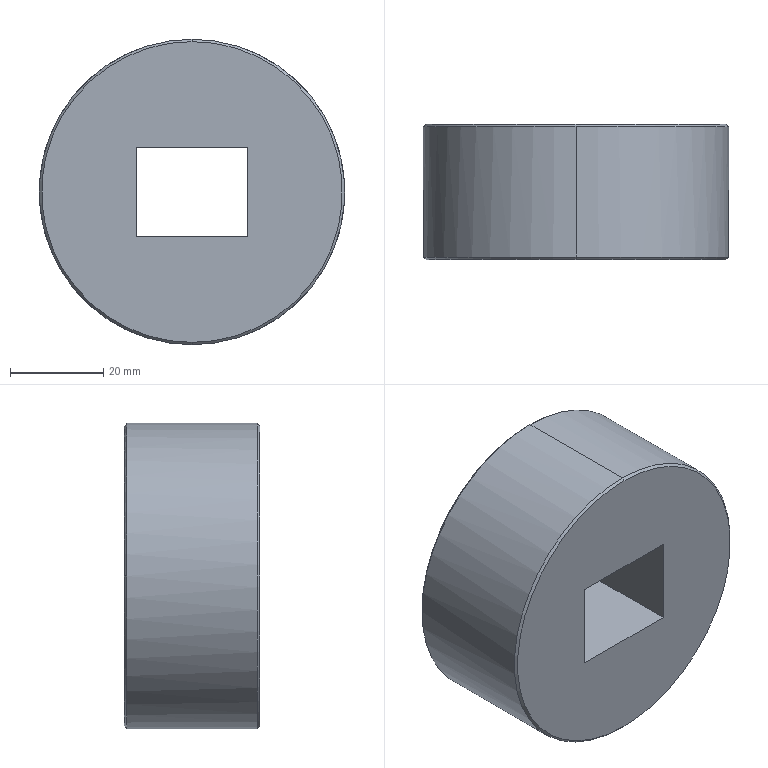Part | STEP file | _X2_4e007ea751859f7f5708_X0_MFB060_2.STEP.STEP | 1 solid | 12 faces | box 65.5 x 29 x 65.5 mm | volume 84346 mm3 | plane 6 | cone 4 | cylinder 2 | commonest cylinder face diameters 65.5 x2
STEP:
#1=CARTESIAN_POINT('',(32.75,28.5,0.));
#2=VERTEX_POINT('',#1);
#3=CARTESIAN_POINT('',(0.,28.5,32.75));
#4=VERTEX_POINT('',#3);
#5=CARTESIAN_POINT('',(0.,28.5,0.));
#6=DIRECTION('',(0.,-1.,0.));
#7=DIRECTION('',(0.,0.,-1.));
#8=AXIS2_PLACEMENT_3D('',#5,#6,#7);
#9=CIRCLE('',#8,32.75);
#10=EDGE_CURVE('',#2,#4,#9,.T.);
#11=ORIENTED_EDGE('',*,*,#10,.T.);
#12=CARTESIAN_POINT('',(0.,0.5,32.75));
#13=VERTEX_POINT('',#12);
#14=CARTESIAN_POINT('',(0.,29.,32.75));
#15=DIRECTION('',(0.,-1.,0.));
#16=VECTOR('',#15,1000.);
#17=LINE('',#14,#16);
#18=EDGE_CURVE('',#4,#13,#17,.T.);
#19=ORIENTED_EDGE('',*,*,#18,.T.);
#20=CARTESIAN_POINT('',(0.,0.5,-32.75));
#21=VERTEX_POINT('',#20);
#22=CARTESIAN_POINT('',(0.,0.5,0.));
#23=DIRECTION('',(0.,1.,0.));
#24=DIRECTION('',(0.,0.,-1.));
#25=AXIS2_PLACEMENT_3D('',#22,#23,#24);
#26=CIRCLE('',#25,32.75);
#27=EDGE_CURVE('',#13,#21,#26,.T.);
#28=ORIENTED_EDGE('',*,*,#27,.T.);
#29=CARTESIAN_POINT('',(0.,28.5,-32.75));
#30=VERTEX_POINT('',#29);
#31=CARTESIAN_POINT('',(0.,29.,-32.75));
#32=DIRECTION('',(0.,-1.,0.));
#33=VECTOR('',#32,1000.);
#34=LINE('',#31,#33);
#35=EDGE_CURVE('',#30,#21,#34,.T.);
#36=ORIENTED_EDGE('',*,*,#35,.F.);
#37=CARTESIAN_POINT('',(0.,28.5,0.));
#38=DIRECTION('',(0.,-1.,0.));
#39=DIRECTION('',(0.,0.,-1.));
#40=AXIS2_PLACEMENT_3D('',#37,#38,#39);
#41=CIRCLE('',#40,32.75);
#42=EDGE_CURVE('',#30,#2,#41,.T.);
#43=ORIENTED_EDGE('',*,*,#42,.T.);
#44=EDGE_LOOP('',(#11,#19,#28,#36,#43));
#45=FACE_OUTER_BOUND('',#44,.T.);
#46=CARTESIAN_POINT('',(0.,29.,0.));
#47=DIRECTION('',(0.,-1.,0.));
#48=DIRECTION('',(0.,0.,-1.));
#49=AXIS2_PLACEMENT_3D('',#46,#47,#48);
#50=CYLINDRICAL_SURFACE('',#49,32.75);
#51=ADVANCED_FACE('',(#45),#50,.T.);
#52=CARTESIAN_POINT('',(0.,0.,32.25));
#53=VERTEX_POINT('',#52);
#54=CARTESIAN_POINT('',(0.,0.,-32.25));
#55=VERTEX_POINT('',#54);
#56=CARTESIAN_POINT('',(0.,0.,0.));
#57=DIRECTION('',(0.,1.,0.));
#58=DIRECTION('',(0.,0.,1.));
#59=AXIS2_PLACEMENT_3D('',#56,#57,#58);
#60=CIRCLE('',#59,32.25);
#61=EDGE_CURVE('',#53,#55,#60,.T.);
#62=ORIENTED_EDGE('',*,*,#61,.T.);
#63=CARTESIAN_POINT('',(0.,0.5,-32.75));
#64=DIRECTION('',(0.,0.7071,-0.7071));
#65=VECTOR('',#64,1000.);
#66=LINE('',#63,#65);
#67=EDGE_CURVE('',#55,#21,#66,.T.);
#68=ORIENTED_EDGE('',*,*,#67,.T.);
#69=ORIENTED_EDGE('',*,*,#27,.F.);
#70=CARTESIAN_POINT('',(0.,0.5,32.75));
#71=DIRECTION('',(0.,0.7071,0.7071));
#72=VECTOR('',#71,1000.);
#73=LINE('',#70,#72);
#74=EDGE_CURVE('',#53,#13,#73,.T.);
#75=ORIENTED_EDGE('',*,*,#74,.F.);
#76=EDGE_LOOP('',(#62,#68,#69,#75));
#77=FACE_OUTER_BOUND('',#76,.T.);
#78=CARTESIAN_POINT('',(0.,0.5,0.));
#79=DIRECTION('',(0.,1.,0.));
#80=DIRECTION('',(0.,0.,1.));
#81=AXIS2_PLACEMENT_3D('',#78,#79,#80);
#82=CONICAL_SURFACE('',#81,32.75,0.7854);
#83=ADVANCED_FACE('',(#77),#82,.T.);
#84=CARTESIAN_POINT('',(32.25,29.,0.));
#85=VERTEX_POINT('',#84);
#86=CARTESIAN_POINT('',(-32.25,29.,0.));
#87=VERTEX_POINT('',#86);
#88=CARTESIAN_POINT('',(0.,29.,0.));
#89=DIRECTION('',(0.,-1.,0.));
#90=DIRECTION('',(1.,0.,0.));
#91=AXIS2_PLACEMENT_3D('',#88,#89,#90);
#92=CIRCLE('',#91,32.25);
#93=EDGE_CURVE('',#85,#87,#92,.T.);
#94=ORIENTED_EDGE('',*,*,#93,.T.);
#95=CARTESIAN_POINT('',(-32.75,28.5,0.));
#96=VERTEX_POINT('',#95);
#97=CARTESIAN_POINT('',(-32.75,28.5,0.));
#98=DIRECTION('',(-0.7071,-0.7071,0.));
#99=VECTOR('',#98,1000.);
#100=LINE('',#97,#99);
#101=EDGE_CURVE('',#87,#96,#100,.T.);
#102=ORIENTED_EDGE('',*,*,#101,.T.);
#103=CARTESIAN_POINT('',(0.,28.5,0.));
#104=DIRECTION('',(0.,-1.,0.));
#105=DIRECTION('',(0.,0.,-1.));
#106=AXIS2_PLACEMENT_3D('',#103,#104,#105);
#107=CIRCLE('',#106,32.75);
#108=EDGE_CURVE('',#4,#96,#107,.T.);
#109=ORIENTED_EDGE('',*,*,#108,.F.);
#110=ORIENTED_EDGE('',*,*,#10,.F.);
#111=CARTESIAN_POINT('',(32.75,28.5,0.));
#112=DIRECTION('',(0.7071,-0.7071,0.));
#113=VECTOR('',#112,1000.);
#114=LINE('',#111,#113);
#115=EDGE_CURVE('',#85,#2,#114,.T.);
#116=ORIENTED_EDGE('',*,*,#115,.F.);
#117=EDGE_LOOP('',(#94,#102,#109,#110,#116));
#118=FACE_OUTER_BOUND('',#117,.T.);
#119=CARTESIAN_POINT('',(0.,28.5,0.));
#120=DIRECTION('',(0.,-1.,0.));
#121=DIRECTION('',(1.,0.,0.));
#122=AXIS2_PLACEMENT_3D('',#119,#120,#121);
#123=CONICAL_SURFACE('',#122,32.75,0.7854);
#124=ADVANCED_FACE('',(#118),#123,.T.);
#125=ORIENTED_EDGE('',*,*,#18,.F.);
#126=ORIENTED_EDGE('',*,*,#108,.T.);
#127=CARTESIAN_POINT('',(0.,28.5,0.));
#128=DIRECTION('',(0.,-1.,0.));
#129=DIRECTION('',(0.,0.,-1.));
#130=AXIS2_PLACEMENT_3D('',#127,#128,#129);
#131=CIRCLE('',#130,32.75);
#132=EDGE_CURVE('',#96,#30,#131,.T.);
#133=ORIENTED_EDGE('',*,*,#132,.T.);
#134=ORIENTED_EDGE('',*,*,#35,.T.);
#135=CARTESIAN_POINT('',(0.,0.5,0.));
#136=DIRECTION('',(0.,1.,0.));
#137=DIRECTION('',(0.,0.,-1.));
#138=AXIS2_PLACEMENT_3D('',#135,#136,#137);
#139=CIRCLE('',#138,32.75);
#140=EDGE_CURVE('',#21,#13,#139,.T.);
#141=ORIENTED_EDGE('',*,*,#140,.T.);
#142=EDGE_LOOP('',(#125,#126,#133,#134,#141));
#143=FACE_OUTER_BOUND('',#142,.T.);
#144=CARTESIAN_POINT('',(0.,29.,0.));
#145=DIRECTION('',(0.,-1.,0.));
#146=DIRECTION('',(0.,0.,-1.));
#147=AXIS2_PLACEMENT_3D('',#144,#145,#146);
#148=CYLINDRICAL_SURFACE('',#147,32.75);
#149=ADVANCED_FACE('',(#143),#148,.T.);
#150=ORIENTED_EDGE('',*,*,#67,.F.);
#151=CARTESIAN_POINT('',(0.,0.,0.));
#152=DIRECTION('',(0.,1.,0.));
#153=DIRECTION('',(0.,0.,1.));
#154=AXIS2_PLACEMENT_3D('',#151,#152,#153);
#155=CIRCLE('',#154,32.25);
#156=EDGE_CURVE('',#55,#53,#155,.T.);
#157=ORIENTED_EDGE('',*,*,#156,.T.);
#158=ORIENTED_EDGE('',*,*,#74,.T.);
#159=ORIENTED_EDGE('',*,*,#140,.F.);
#160=EDGE_LOOP('',(#150,#157,#158,#159));
#161=FACE_OUTER_BOUND('',#160,.T.);
#162=CARTESIAN_POINT('',(0.,0.5,0.));
#163=DIRECTION('',(0.,1.,0.));
#164=DIRECTION('',(0.,0.,1.));
#165=AXIS2_PLACEMENT_3D('',#162,#163,#164);
#166=CONICAL_SURFACE('',#165,32.75,0.7854);
#167=ADVANCED_FACE('',(#161),#166,.T.);
#168=ORIENTED_EDGE('',*,*,#101,.F.);
#169=CARTESIAN_POINT('',(0.,29.,0.));
#170=DIRECTION('',(0.,-1.,0.));
#171=DIRECTION('',(1.,0.,0.));
#172=AXIS2_PLACEMENT_3D('',#169,#170,#171);
#173=CIRCLE('',#172,32.25);
#174=EDGE_CURVE('',#87,#85,#173,.T.);
#175=ORIENTED_EDGE('',*,*,#174,.T.);
#176=ORIENTED_EDGE('',*,*,#115,.T.);
#177=ORIENTED_EDGE('',*,*,#42,.F.);
#178=ORIENTED_EDGE('',*,*,#132,.F.);
#179=EDGE_LOOP('',(#168,#175,#176,#177,#178));
#180=FACE_OUTER_BOUND('',#179,.T.);
#181=CARTESIAN_POINT('',(0.,28.5,0.));
#182=DIRECTION('',(0.,-1.,0.));
#183=DIRECTION('',(1.,0.,0.));
#184=AXIS2_PLACEMENT_3D('',#181,#182,#183);
#185=CONICAL_SURFACE('',#184,32.75,0.7854);
#186=ADVANCED_FACE('',(#180),#185,.T.);
#187=ORIENTED_EDGE('',*,*,#61,.F.);
#188=ORIENTED_EDGE('',*,*,#156,.F.);
#189=EDGE_LOOP('',(#187,#188));
#190=FACE_OUTER_BOUND('',#189,.T.);
#191=CARTESIAN_POINT('',(11.93,0.,-9.625));
#192=VERTEX_POINT('',#191);
#193=CARTESIAN_POINT('',(11.93,0.,9.625));
#194=VERTEX_POINT('',#193);
#195=CARTESIAN_POINT('',(11.93,0.,0.));
#196=DIRECTION('',(0.,0.,1.));
#197=VECTOR('',#196,1000.);
#198=LINE('',#195,#197);
#199=EDGE_CURVE('',#192,#194,#198,.T.);
#200=ORIENTED_EDGE('',*,*,#199,.F.);
#201=CARTESIAN_POINT('',(-11.93,0.,-9.625));
#202=VERTEX_POINT('',#201);
#203=CARTESIAN_POINT('',(0.,0.,-9.625));
#204=DIRECTION('',(1.,0.,0.));
#205=VECTOR('',#204,1000.);
#206=LINE('',#203,#205);
#207=EDGE_CURVE('',#202,#192,#206,.T.);
#208=ORIENTED_EDGE('',*,*,#207,.F.);
#209=CARTESIAN_POINT('',(-11.93,0.,9.625));
#210=VERTEX_POINT('',#209);
#211=CARTESIAN_POINT('',(-11.93,0.,0.));
#212=DIRECTION('',(0.,0.,-1.));
#213=VECTOR('',#212,1000.);
#214=LINE('',#211,#213);
#215=EDGE_CURVE('',#210,#202,#214,.T.);
#216=ORIENTED_EDGE('',*,*,#215,.F.);
#217=CARTESIAN_POINT('',(0.,0.,9.625));
#218=DIRECTION('',(-1.,0.,0.));
#219=VECTOR('',#218,1000.);
#220=LINE('',#217,#219);
#221=EDGE_CURVE('',#194,#210,#220,.T.);
#222=ORIENTED_EDGE('',*,*,#221,.F.);
#223=EDGE_LOOP('',(#200,#208,#216,#222));
#224=FACE_BOUND('',#223,.T.);
#225=CARTESIAN_POINT('',(0.,0.,0.));
#226=DIRECTION('',(0.,1.,0.));
#227=DIRECTION('',(0.,0.,1.));
#228=AXIS2_PLACEMENT_3D('',#225,#226,#227);
#229=PLANE('',#228);
#230=ADVANCED_FACE('',(#190,#224),#229,.F.);
#231=ORIENTED_EDGE('',*,*,#93,.F.);
#232=ORIENTED_EDGE('',*,*,#174,.F.);
#233=EDGE_LOOP('',(#231,#232));
#234=FACE_OUTER_BOUND('',#233,.T.);
#235=CARTESIAN_POINT('',(-11.93,29.,9.625));
#236=VERTEX_POINT('',#235);
#237=CARTESIAN_POINT('',(-11.93,29.,-9.625));
#238=VERTEX_POINT('',#237);
#239=CARTESIAN_POINT('',(-11.93,29.,0.));
#240=DIRECTION('',(0.,0.,-1.));
#241=VECTOR('',#240,1000.);
#242=LINE('',#239,#241);
#243=EDGE_CURVE('',#236,#238,#242,.T.);
#244=ORIENTED_EDGE('',*,*,#243,.T.);
#245=CARTESIAN_POINT('',(11.93,29.,-9.625));
#246=VERTEX_POINT('',#245);
#247=CARTESIAN_POINT('',(0.,29.,-9.625));
#248=DIRECTION('',(1.,0.,0.));
#249=VECTOR('',#248,1000.);
#250=LINE('',#247,#249);
#251=EDGE_CURVE('',#238,#246,#250,.T.);
#252=ORIENTED_EDGE('',*,*,#251,.T.);
#253=CARTESIAN_POINT('',(11.93,29.,9.625));
#254=VERTEX_POINT('',#253);
#255=CARTESIAN_POINT('',(11.93,29.,0.));
#256=DIRECTION('',(0.,0.,1.));
#257=VECTOR('',#256,1000.);
#258=LINE('',#255,#257);
#259=EDGE_CURVE('',#246,#254,#258,.T.);
#260=ORIENTED_EDGE('',*,*,#259,.T.);
#261=CARTESIAN_POINT('',(0.,29.,9.625));
#262=DIRECTION('',(-1.,0.,0.));
#263=VECTOR('',#262,1000.);
#264=LINE('',#261,#263);
#265=EDGE_CURVE('',#254,#236,#264,.T.);
#266=ORIENTED_EDGE('',*,*,#265,.T.);
#267=EDGE_LOOP('',(#244,#252,#260,#266));
#268=FACE_BOUND('',#267,.T.);
#269=CARTESIAN_POINT('',(0.,29.,0.));
#270=DIRECTION('',(0.,1.,0.));
#271=DIRECTION('',(0.,0.,1.));
#272=AXIS2_PLACEMENT_3D('',#269,#270,#271);
#273=PLANE('',#272);
#274=ADVANCED_FACE('',(#234,#268),#273,.T.);
#275=CARTESIAN_POINT('',(11.93,0.,9.625));
#276=DIRECTION('',(0.,1.,0.));
#277=VECTOR('',#276,1000.);
#278=LINE('',#275,#277);
#279=EDGE_CURVE('',#194,#254,#278,.T.);
#280=ORIENTED_EDGE('',*,*,#279,.F.);
#281=ORIENTED_EDGE('',*,*,#221,.T.);
#282=CARTESIAN_POINT('',(-11.93,0.,9.625));
#283=DIRECTION('',(0.,-1.,0.));
#284=VECTOR('',#283,1000.);
#285=LINE('',#282,#284);
#286=EDGE_CURVE('',#236,#210,#285,.T.);
#287=ORIENTED_EDGE('',*,*,#286,.F.);
#288=ORIENTED_EDGE('',*,*,#265,.F.);
#289=EDGE_LOOP('',(#280,#281,#287,#288));
#290=FACE_OUTER_BOUND('',#289,.T.);
#291=CARTESIAN_POINT('',(-11.93,0.,9.625));
#292=DIRECTION('',(0.,0.,1.));
#293=DIRECTION('',(1.,0.,0.));
#294=AXIS2_PLACEMENT_3D('',#291,#292,#293);
#295=PLANE('',#294);
#296=ADVANCED_FACE('',(#290),#295,.F.);
#297=CARTESIAN_POINT('',(11.93,0.,-9.625));
#298=DIRECTION('',(0.,1.,0.));
#299=VECTOR('',#298,1000.);
#300=LINE('',#297,#299);
#301=EDGE_CURVE('',#192,#246,#300,.T.);
#302=ORIENTED_EDGE('',*,*,#301,.F.);
#303=ORIENTED_EDGE('',*,*,#199,.T.);
#304=ORIENTED_EDGE('',*,*,#279,.T.);
#305=ORIENTED_EDGE('',*,*,#259,.F.);
#306=EDGE_LOOP('',(#302,#303,#304,#305));
#307=FACE_OUTER_BOUND('',#306,.T.);
#308=CARTESIAN_POINT('',(11.93,0.,-9.625));
#309=DIRECTION('',(1.,0.,0.));
#310=DIRECTION('',(0.,0.,-1.));
#311=AXIS2_PLACEMENT_3D('',#308,#309,#310);
#312=PLANE('',#311);
#313=ADVANCED_FACE('',(#307),#312,.F.);
#314=CARTESIAN_POINT('',(-11.93,0.,-9.625));
#315=DIRECTION('',(0.,1.,0.));
#316=VECTOR('',#315,1000.);
#317=LINE('',#314,#316);
#318=EDGE_CURVE('',#202,#238,#317,.T.);
#319=ORIENTED_EDGE('',*,*,#318,.F.);
#320=ORIENTED_EDGE('',*,*,#207,.T.);
#321=ORIENTED_EDGE('',*,*,#301,.T.);
#322=ORIENTED_EDGE('',*,*,#251,.F.);
#323=EDGE_LOOP('',(#319,#320,#321,#322));
#324=FACE_OUTER_BOUND('',#323,.T.);
#325=CARTESIAN_POINT('',(-11.93,0.,-9.625));
#326=DIRECTION('',(0.,0.,-1.));
#327=DIRECTION('',(-1.,0.,0.));
#328=AXIS2_PLACEMENT_3D('',#325,#326,#327);
#329=PLANE('',#328);
#330=ADVANCED_FACE('',(#324),#329,.F.);
#331=ORIENTED_EDGE('',*,*,#286,.T.);
#332=ORIENTED_EDGE('',*,*,#215,.T.);
#333=ORIENTED_EDGE('',*,*,#318,.T.);
#334=ORIENTED_EDGE('',*,*,#243,.F.);
#335=EDGE_LOOP('',(#331,#332,#333,#334));
#336=FACE_OUTER_BOUND('',#335,.T.);
#337=CARTESIAN_POINT('',(-11.93,0.,-9.625));
#338=DIRECTION('',(-1.,0.,0.));
#339=DIRECTION('',(0.,0.,1.));
#340=AXIS2_PLACEMENT_3D('',#337,#338,#339);
#341=PLANE('',#340);
#342=ADVANCED_FACE('',(#336),#341,.F.);
#343=CLOSED_SHELL('',(#51,#83,#124,#149,#167,#186,#230,#274,#296,#313,#330,#342));
#344=MANIFOLD_SOLID_BREP('',#343);
#345=CARTESIAN_POINT('',(0.,0.,0.));
#346=DIRECTION('',(0.,0.,1.));
#347=DIRECTION('',(1.,0.,0.));
#348=AXIS2_PLACEMENT_3D('',#345,#346,#347);
#349=(LENGTH_UNIT()NAMED_UNIT(*)SI_UNIT(.MILLI.,.METRE.));
#350=UNCERTAINTY_MEASURE_WITH_UNIT(LENGTH_MEASURE(0.00001),#349,'','');
#351=(NAMED_UNIT(*)PLANE_ANGLE_UNIT()SI_UNIT($,.RADIAN.));
#352=(NAMED_UNIT(*)SI_UNIT($,.STERADIAN.)SOLID_ANGLE_UNIT());
#353=(GEOMETRIC_REPRESENTATION_CONTEXT(3)GLOBAL_UNCERTAINTY_ASSIGNED_CONTEXT((#350))GLOBAL_UNIT_ASSIGNED_CONTEXT((#349,#351,#352))REPRESENTATION_CONTEXT('',''));
#354=ADVANCED_BREP_SHAPE_REPRESENTATION('',(#344,#348),#353);